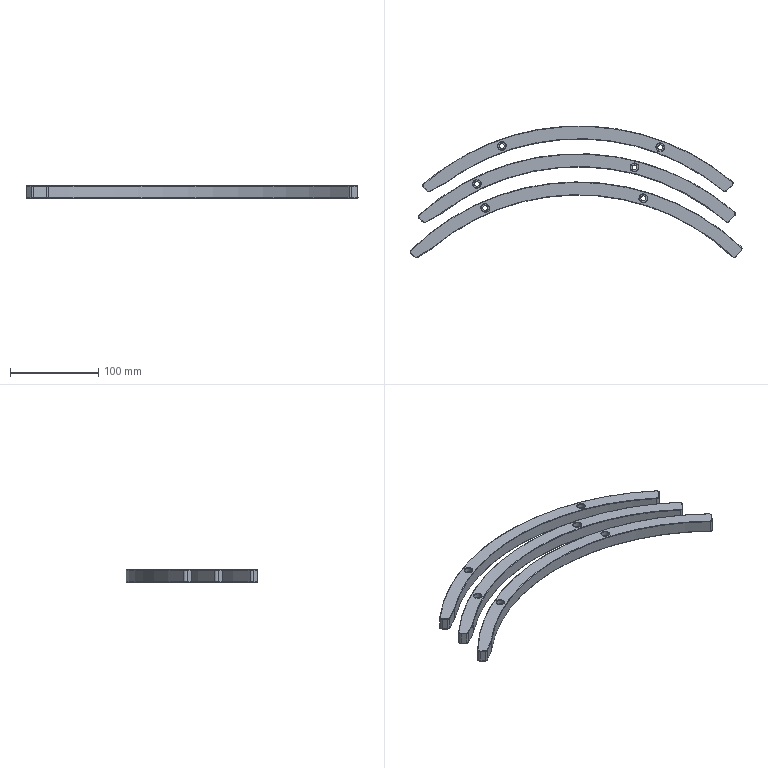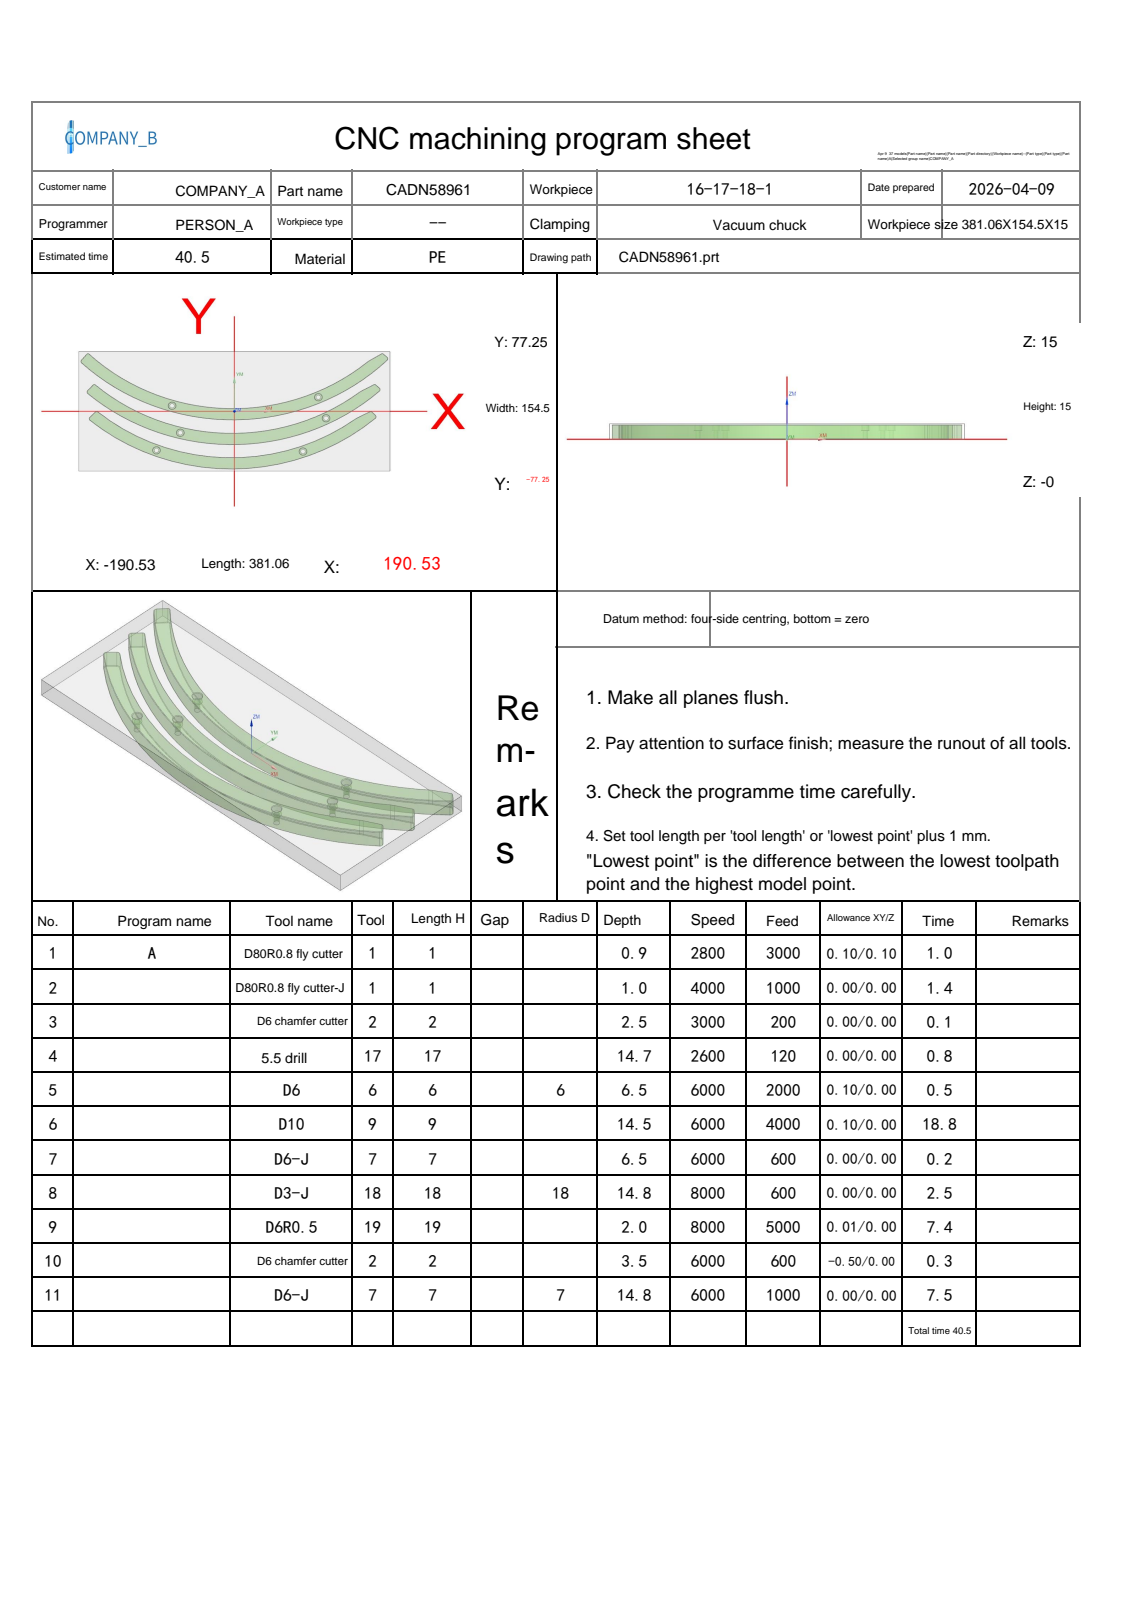NC program | NX | posted by the shop | part box 376.065 x 149.521 x 14 mm
Lines 2624 to 3929 of 3929:
N9 T19 M06
(D6R0.5  D=6. R=0.5 H=19 ce=0.01 di=0.00)
(MAX_Z=25. MIN_Z=13. Time=7.39M)
G00 G90 G54 X168.35 Y73.543 M03 S8000
G43 H19 Z25.
M08
Z14.484
G01 Z13.984 F5000.
X169.888 Y70.967
X178.897 Y76.346
G02 X181.043 Y76.938 I2.146 J-3.595
X183.776 Y75.923 I0.0 J-4.187
G01 X188.418 Y71.923
G02 X190.219 Y67.994 I-3.386 J-3.929
X188.662 Y64.289 I-5.187 J0.0
X-1.828 Y-13.478 I-190.491 J194.419
X-188.591 Y60.706 I0.0 J272.187
X-190.219 Y64.479 I3.559 J3.773
X-188.962 Y67.865 I5.187 J0.0
G01 X-182.395 Y75.485
G02 X-179.224 Y76.939 I3.172 J-2.733
X-176.334 Y75.781 I0.0 J-4.187
G03 X-1.828 Y5.895 I174.505 J182.927
X161.04 Y65.348 I0.0 J252.813
G02 X163.96 Y67.429 I14.293 J-16.969
G01 X169.888 Y70.967
X169.857 Y71.018 Z13.972
X169.834 Y71.058 Z13.959
X163.906 Y67.519
G03 X160.972 Y65.428 I11.427 J-19.14
G02 X-1.828 Y6.001 I-162.8 J193.281
X-176.257 Y75.854 I0.0 J252.708
G03 X-179.224 Y77.044 I-2.966 J-3.102
X-182.475 Y75.553 I0.0 J-4.292
G01 X-189.041 Y67.933
G03 X-190.324 Y64.479 I4.009 J-3.454
X-188.664 Y60.629 I5.292 J0.0
X-1.828 Y-13.583 I186.835 J198.079
X188.736 Y64.214 I0.0 J272.292
X190.324 Y67.994 I-3.704 J3.78
X188.487 Y72.003 I-5.292 J0.0
G01 X183.845 Y76.003
G03 X181.043 Y77.043 I-2.802 J-3.251
X178.843 Y76.437 I0.0 J-4.292
G01 X169.834 Y71.058
X169.806 Y71.103 Z13.942
X169.783 Y71.142 Z13.925
X178.793 Y76.521
G02 X181.043 Y77.142 I2.251 J-3.77
X183.909 Y76.077 I0.0 J-4.39
G01 X188.551 Y72.078
G02 X190.423 Y67.994 I-3.519 J-4.083
X188.805 Y64.144 I-5.39 J0.0
X-1.828 Y-13.682 I-190.633 J194.565
X-188.731 Y60.558 I0.0 J272.39
X-190.423 Y64.479 I3.699 J3.921
X-189.116 Y67.997 I5.39 J0.0
G01 X-182.55 Y75.618
G02 X-179.224 Y77.142 I3.326 J-2.866
X-176.193 Y75.929 I0.0 J-4.39
G03 X-1.828 Y6.099 I174.365 J182.78
X160.909 Y65.503 I0.0 J252.61
G02 X163.856 Y67.603 I14.425 J-17.125
G01 X169.783 Y71.142
X169.758 Y71.184 Z13.903
X169.736 Y71.221 Z13.881
X163.808 Y67.683
G03 X160.849 Y65.574 I11.525 J-19.304
G02 X-1.828 Y6.191 I-162.678 J193.135
X-176.129 Y75.995 I0.0 J252.517
G03 X-179.224 Y77.235 I-3.094 J-3.244
X-182.62 Y75.678 I0.0 J-4.483
G01 X-189.186 Y68.058
G03 X-190.515 Y64.479 I4.153 J-3.579
X-188.794 Y60.49 I5.483 J0.0
X-1.828 Y-13.774 I186.966 J198.218
X188.869 Y64.078 I0.0 J272.483
X190.515 Y67.994 I-3.837 J3.916
X188.611 Y72.148 I-5.483 J0.0
G01 X183.969 Y76.147
G03 X181.043 Y77.234 I-2.926 J-3.396
X178.745 Y76.6 I0.0 J-4.483
G01 X169.736 Y71.221
X169.712 Y71.261 Z13.855
X169.691 Y71.296 Z13.829
X178.701 Y76.675
G02 X181.043 Y77.321 I2.342 J-3.924
X184.026 Y76.213 I0.0 J-4.57
G01 X188.668 Y72.214
G02 X190.602 Y67.994 I-3.636 J-4.219
X188.93 Y64.016 I-5.57 J0.0
X-1.828 Y-13.861 I-190.759 J194.693
X-188.854 Y60.427 I0.0 J272.57
X-190.602 Y64.479 I3.822 J4.052
X-189.252 Y68.115 I5.57 J0.0
G01 X-182.685 Y75.735
G02 X-179.224 Y77.322 I3.462 J-2.983
X-176.069 Y76.058 I0.0 J-4.57
G03 X-1.828 Y6.278 I174.241 J182.65
X160.793 Y65.641 I0.0 J252.43
G02 X163.764 Y67.757 I14.54 J-17.262
G01 X169.691 Y71.296
X169.669 Y71.333 Z13.798
X169.65 Y71.366 Z13.768
X163.722 Y67.827
G03 X160.741 Y65.703 I11.611 J-19.448
G02 X-1.828 Y6.359 I-162.57 J193.006
X-176.014 Y76.117 I0.0 J252.35
G03 X-179.224 Y77.402 I-3.21 J-3.365
X-182.747 Y75.788 I0.0 J-4.65
G01 X-189.313 Y68.167
G03 X-190.683 Y64.479 I4.281 J-3.688
X-188.91 Y60.368 I5.65 J0.0
X-1.828 Y-13.942 I187.081 J198.34
X188.987 Y63.958 I0.0 J272.65
X190.683 Y67.994 I-3.954 J4.036
X188.721 Y72.275 I-5.65 J0.0
G01 X184.079 Y76.274
G03 X181.043 Y77.402 I-3.036 J-3.523
X178.659 Y76.744 I0.0 J-4.65
G01 X169.65 Y71.366
X169.63 Y71.399 Z13.734
X169.612 Y71.429 Z13.7
X178.622 Y76.808
G02 X181.043 Y77.476 I2.422 J-4.057
X184.127 Y76.331 I0.0 J-4.724
G01 X188.769 Y72.331
G02 X190.757 Y67.994 I-3.737 J-4.337
X189.039 Y63.905 I-5.724 J0.0
X-1.828 Y-14.016 I-190.867 J194.803
X-188.96 Y60.314 I0.0 J272.724
X-190.757 Y64.479 I3.928 J4.164
X-189.369 Y68.216 I5.724 J0.0
G01 X-182.803 Y75.836
G02 X-179.224 Y77.476 I3.579 J-3.084
X-175.963 Y76.17 I0.0 J-4.724
G03 X-1.828 Y6.433 I174.134 J182.538
X160.694 Y65.759 I0.0 J252.276
G02 X163.685 Y67.89 I14.639 J-17.381
G01 X169.612 Y71.429
X169.594 Y71.459 Z13.662
X169.578 Y71.486 Z13.624
X163.65 Y67.948
G03 X160.651 Y65.81 I11.683 J-19.569
G02 X-1.828 Y6.5 I-162.479 J192.899
X-175.917 Y76.219 I0.0 J252.209
G03 X-179.224 Y77.543 I-3.307 J-3.467
X-182.853 Y75.879 I0.0 J-4.791
G01 X-189.419 Y68.259
G03 X-190.824 Y64.479 I4.387 J-3.78
X-189.006 Y60.266 I5.791 J0.0
X-1.828 Y-14.082 I187.178 J198.443
X189.085 Y63.858 I0.0 J272.791
X190.824 Y67.994 I-4.053 J4.136
X188.813 Y72.381 I-5.791 J0.0
G01 X184.171 Y76.381
G03 X181.043 Y77.543 I-3.128 J-3.63
X178.587 Y76.865 I0.0 J-4.791
G01 X169.578 Y71.486
X169.562 Y71.513 Z13.584
X169.548 Y71.537 Z13.543
X178.557 Y76.916
G02 X181.043 Y77.601 I2.486 J-4.164
X184.209 Y76.425 I0.0 J-4.85
G01 X188.851 Y72.426
G02 X190.882 Y67.994 I-3.819 J-4.432
X189.126 Y63.816 I-5.85 J0.0
X-1.828 Y-14.141 I-190.955 J194.893
X-189.046 Y60.223 I0.0 J272.85
X-190.882 Y64.479 I4.014 J4.255
X-189.464 Y68.297 I5.85 J0.0
G01 X-182.898 Y75.918
G02 X-179.224 Y77.602 I3.674 J-3.166
X-175.876 Y76.261 I0.0 J-4.85
G03 X-1.828 Y6.559 I174.048 J182.448
X160.613 Y65.855 I0.0 J252.15
G02 X163.62 Y67.998 I14.72 J-17.476
G01 X169.548 Y71.537
X169.534 Y71.559 Z13.499
X169.522 Y71.58 Z13.456
X163.594 Y68.041
G03 X160.58 Y65.893 I11.739 J-19.662
G02 X-1.828 Y6.609 I-162.409 J192.815
X-175.841 Y76.297 I0.0 J252.1
G03 X-179.224 Y77.652 I-3.382 J-3.545
X-182.936 Y75.95 I0.0 J-4.9
G01 X-189.502 Y68.33
G03 X-190.932 Y64.479 I4.47 J-3.851
X-189.081 Y60.187 I5.9 J0.0
X-1.828 Y-14.191 I187.252 J198.522
X189.162 Y63.78 I0.0 J272.9
X190.932 Y67.994 I-4.129 J4.214
X188.884 Y72.464 I-5.9 J0.0
G01 X184.242 Y76.463
G03 X181.043 Y77.651 I-3.199 J-3.712
X178.532 Y76.959 I0.0 J-4.9
G01 X169.522 Y71.58
X169.511 Y71.599 Z13.41
X169.501 Y71.615 Z13.365
X178.51 Y76.994
G02 X181.043 Y77.693 I2.533 J-4.243
X184.269 Y76.495 I0.0 J-4.941
G01 X188.911 Y72.495
G02 X190.974 Y67.994 I-3.878 J-4.501
X189.19 Y63.75 I-5.941 J0.0
X-1.828 Y-14.232 I-191.019 J194.958
X-189.109 Y60.157 I0.0 J272.941
X-190.974 Y64.479 I4.077 J4.322
X-189.533 Y68.357 I5.941 J0.0
G01 X-182.967 Y75.977
G02 X-179.224 Y77.693 I3.743 J-3.225
X-175.813 Y76.327 I0.0 J-4.941
G03 X-1.828 Y6.65 I173.985 J182.382
X160.554 Y65.925 I0.0 J252.059
G02 X163.573 Y68.076 I14.779 J-17.546
G01 X169.501 Y71.615
X169.492 Y71.629 Z13.319
X169.485 Y71.641 Z13.274
X163.558 Y68.103
G03 X160.534 Y65.948 I11.776 J-19.724
G02 X-1.828 Y6.681 I-162.363 J192.76
X-175.792 Y76.349 I0.0 J252.028
G03 X-179.224 Y77.724 I-3.432 J-3.597
X-182.99 Y75.997 I0.0 J-4.972
G01 X-189.556 Y68.377
G03 X-191.004 Y64.479 I4.524 J-3.898
X-189.13 Y60.135 I5.972 J0.0
X-1.828 Y-14.263 I187.302 J198.574
X189.212 Y63.728 I0.0 J272.972
X191.004 Y67.994 I-4.179 J4.266
X188.931 Y72.518 I-5.972 J0.0
G01 X184.289 Y76.518
G03 X181.043 Y77.723 I-3.245 J-3.766
X178.495 Y77.02 I0.0 J-4.972
G01 X169.485 Y71.641
X169.479 Y71.652 Z13.228
X169.474 Y71.66 Z13.182
X178.484 Y77.039
G02 X181.043 Y77.745 I2.56 J-4.287
X184.303 Y76.534 I0.0 J-4.993
G01 X188.945 Y72.534
G02 X191.026 Y67.994 I-3.912 J-4.54
X189.227 Y63.713 I-5.993 J0.0
X-1.828 Y-14.285 I-191.055 J194.995
X-189.145 Y60.119 I0.0 J272.993
X-191.026 Y64.479 I4.112 J4.36
X-189.573 Y68.391 I5.993 J0.0
G01 X-183.006 Y76.011
G02 X-179.224 Y77.745 I3.783 J-3.259
X-175.777 Y76.365 I0.0 J-4.993
G03 X-1.828 Y6.702 I173.949 J182.344
X160.52 Y65.965 I0.0 J252.007
G02 X163.547 Y68.121 I14.813 J-17.586
G01 X169.474 Y71.66
X169.47 Y71.666 Z13.137
X169.468 Y71.671 Z13.091
X163.54 Y68.132
G03 X160.512 Y65.974 I11.793 J-19.753
G02 X-1.828 Y6.715 I-162.341 J192.734
X-175.768 Y76.374 I0.0 J251.994
G03 X-179.224 Y77.758 I-3.455 J-3.622
X-183.016 Y76.02 I0.0 J-5.006
G01 X-189.582 Y68.399
G03 X-191.038 Y64.479 I4.55 J-3.92
X-189.153 Y60.11 I6.006 J0.0
X-1.828 Y-14.297 I187.325 J198.599
X189.236 Y63.704 I0.0 J273.006
X191.038 Y67.994 I-4.203 J4.29
X188.953 Y72.544 I-6.006 J0.0
G01 X184.311 Y76.544
G03 X181.043 Y77.757 I-3.268 J-3.792
X178.477 Y77.05 I0.0 J-5.006
G01 X169.468 Y71.671
X169.465 Y71.674 Z13.
X178.476 Y77.054
G02 X179.504 Y77.519 I2.592 J-4.356
X179.713 Y77.582 I1.539 J-4.768
X181.042 Y77.761 I1.329 J-4.834
X184.314 Y76.547 I0.0 J-5.014
G01 X188.787 Y72.692
X189.178 Y72.346
G02 X191.042 Y67.994 I-4.148 J-4.352
X190.464 Y65.422 I-6.013 J0.0
X190.12 Y64.794 I-6.048 J2.91
X189.246 Y63.708 I-5.151 J3.252
X-1.842 Y-14.305 I-191.088 J195.02
X-26.922 Y-13.151 I0.0 J273.034
G01 X-26.934 Y-13.143
X-27.069 Y-13.131
X-30.191 Y-12.824
X-30.437 Y-12.798
X-33.554 Y-12.452
X-36.387 Y-12.105
G02 X-69.081 Y-5.894 I34.769 J272.19
G01 X-69.394 Y-5.808
G02 X-88.032 Y-.339 I68.396 J267.567
G01 X-88.052 Y-.327
X-89.862 Y.282
X-90.101 Y.363
X-91.104 Y.709
X-91.108
G02 X-100.542 Y4.167 I92.07 J265.779
X-109.05 Y7.635 I103.191 J265.362
X-129.387 Y17.331 I107.517 J251.692
X-189.156 Y60.107 I127.592 J241.425
X-190.121 Y61.28 I4.155 J4.397
X-191.042 Y64.479 I5.088 J3.199
X-190.392 Y67.199 I6.01 J0.0
X-189.585 Y68.402 I5.359 J-2.72
G01 X-183.019 Y76.022
G02 X-182.148 Y76.82 I3.795 J-3.27
G01 X-182.059 Y76.882
G02 X-179.224 Y77.762 I2.836 J-4.132
X-175.765 Y76.377 I0.0 J-5.011
G01 X-173.359 Y74.112
X-172.985 Y73.765
G03 X-1.828 Y6.719 I171.157 J184.944
X157.334 Y63.347 I0.0 J251.99
G01 X157.758 Y63.694
X160.63 Y66.078
G02 X163.538 Y68.135 I14.739 J-17.743
G01 X169.465 Y71.674
G00 Z25.
X159.122 Y34.303
Z14.484
G01 Z13.984
X160.545 Y31.663
X169.783 Y36.641
G02 X171.769 Y37.142 I1.986 J-3.686
X174.639 Y36.004 I0.0 J-4.187
G01 X179.1 Y31.804
G02 X180.732 Y28.027 I-3.555 J-3.777
X179.009 Y24.167 I-5.187 J0.0
X-2.761 Y-45.424 I-181.77 J202.596
X-180.995 Y21.049 I0.0 J272.187
X-182.786 Y24.969 I3.396 J3.92
X-181.376 Y28.524 I5.187 J0.0
G01 X-174.544 Y35.782
G02 X-171.495 Y37.099 I3.049 J-2.87
X-168.746 Y36.07 I0.0 J-4.187
G03 X-2.761 Y-26.051 I165.985 J190.692
X151.46 Y26.437 I0.0 J252.813
G02 X154.468 Y28.387 I13.535 J-17.58
G01 X160.545 Y31.663
X160.518 Y31.714 Z13.972
X160.496 Y31.755 Z13.959
X154.419 Y28.48
G03 X151.395 Y26.52 I10.576 J-19.624
G02 X-2.761 Y-25.945 I-154.157 J200.243
X-168.677 Y36.15 I0.0 J252.708
G03 X-171.495 Y37.204 I-2.818 J-3.237
X-174.62 Y35.854 I0.0 J-4.292
G01 X-181.452 Y28.596
G03 X-182.891 Y24.969 I3.853 J-3.627
X-181.064 Y20.969 I5.292 J0.0
X-2.761 Y-45.529 I178.303 J205.794
X179.079 Y24.088 I0.0 J272.292
X180.837 Y28.027 I-3.534 J3.939
X179.172 Y31.881 I-5.292 J0.0
G01 X174.711 Y36.08
G03 X171.769 Y37.247 I-2.942 J-3.125
X169.733 Y36.733 I0.0 J-4.292
G01 X160.496 Y31.755
X160.47 Y31.802 Z13.942
X160.449 Y31.842 Z13.925
X169.686 Y36.82
G02 X171.769 Y37.345 I2.083 J-3.865
X174.778 Y36.152 I0.0 J-4.39
G01 X179.24 Y31.952
G02 X180.935 Y28.027 I-3.694 J-3.925
X179.145 Y24.015 I-5.39 J0.0
X-2.761 Y-45.628 I-181.906 J202.748
X-181.128 Y20.895 I0.0 J272.39
X-182.989 Y24.969 I3.53 J4.074
X-181.524 Y28.663 I5.39 J0.0
G01 X-174.692 Y35.921
G02 X-171.495 Y37.303 I3.197 J-3.009
X-168.613 Y36.224 I0.0 J-4.39
G03 X-2.761 Y-25.847 I165.851 J190.539
X151.335 Y26.598 I0.0 J252.61
G02 X154.372 Y28.567 I13.659 J-17.742
G01 X160.449 Y31.842
X160.426 Y31.885 Z13.903
X160.405 Y31.923 Z13.881
X154.328 Y28.648
G03 X151.279 Y26.671 I10.666 J-19.792
G02 X-2.761 Y-25.755 I-154.04 J200.091
X-168.552 Y36.294 I0.0 J252.517
G03 X-171.495 Y37.395 I-2.943 J-3.381
X-174.759 Y35.985 I0.0 J-4.483
G01 X-181.591 Y28.727
G03 X-183.082 Y24.969 I3.992 J-3.758
X-181.189 Y20.825 I5.483 J0.0
X-2.761 Y-45.72 I178.428 J205.938
X179.207 Y23.946 I0.0 J272.483
X181.028 Y28.027 I-3.661 J4.081
X179.303 Y32.02 I-5.483 J0.0
G01 X174.841 Y36.219
G03 X171.769 Y37.438 I-3.073 J-3.264
X169.642 Y36.901 I0.0 J-4.483
G01 X160.405 Y31.923
X160.383 Y31.964 Z13.855
X160.364 Y32. Z13.829
X169.601 Y36.978
G02 X171.769 Y37.525 I2.168 J-4.023
X174.901 Y36.283 I0.0 J-4.57
G01 X179.363 Y32.083
G02 X181.115 Y28.027 I-3.817 J-4.056
X179.265 Y23.882 I-5.57 J0.0
X-2.761 Y-45.807 I-182.026 J202.881
X-181.246 Y20.759 I0.0 J272.57
X-183.169 Y24.969 I3.647 J4.21
X-181.654 Y28.786 I5.57 J0.0
G01 X-174.822 Y36.044
G02 X-171.495 Y37.482 I3.327 J-3.132
X-168.495 Y36.359 I0.0 J-4.57
G03 X-2.761 Y-25.668 I165.733 J190.404
X151.226 Y26.74 I0.0 J252.43
G02 X154.287 Y28.725 I13.768 J-17.884
G01 X160.364 Y32.
X160.344 Y32.037 Z13.798
X160.325 Y32.071 Z13.768
X154.248 Y28.796
G03 X151.177 Y26.804 I10.746 J-19.939
G02 X-2.761 Y-25.587 I-153.938 J199.958
X-168.442 Y36.42 I0.0 J252.35
G03 X-171.495 Y37.563 I-3.053 J-3.508
X-174.881 Y36.1 I0.0 J-4.65
G01 X-181.713 Y28.842
G03 X-183.249 Y24.969 I4.114 J-3.873
X-181.299 Y20.698 I5.65 J0.0
X-2.761 Y-45.888 I178.538 J206.065
X179.319 Y23.822 I0.0 J272.65
X181.196 Y28.027 I-3.774 J4.206
X179.418 Y32.142 I-5.65 J0.0
G01 X174.956 Y36.341
G03 X171.769 Y37.606 I-3.187 J-3.386
X169.563 Y37.049 I0.0 J-4.65
G01 X160.325 Y32.071
X160.307 Y32.105 Z13.734
X160.29 Y32.136 Z13.7
X169.527 Y37.114
G02 X171.769 Y37.68 I2.241 J-4.159
X175.007 Y36.395 I0.0 J-4.724
G01 X179.469 Y32.196
G02 X181.27 Y28.027 I-3.924 J-4.168
X179.368 Y23.766 I-5.724 J0.0
X-2.761 Y-45.962 I-182.13 J202.996
X-181.347 Y20.642 I0.0 J272.724
X-183.323 Y24.969 I3.748 J4.327
X-181.767 Y28.892 I5.724 J0.0
G01 X-174.935 Y36.15
G02 X-171.495 Y37.637 I3.44 J-3.238
X-168.393 Y36.476 I0.0 J-4.724
G03 X-2.761 Y-25.513 I165.632 J190.287
X151.132 Y26.863 I0.0 J252.276
G02 X154.213 Y28.861 I13.862 J-18.007
G01 X160.29 Y32.136
X160.274 Y32.167 Z13.662
X160.259 Y32.195 Z13.624
X154.182 Y28.919
G03 X151.091 Y26.916 I10.813 J-20.063
G02 X-2.761 Y-25.446 I-153.853 J199.847
X-168.349 Y36.526 I0.0 J252.209
G03 X-171.495 Y37.703 I-3.146 J-3.614
X-174.984 Y36.196 I0.0 J-4.791
G01 X-181.816 Y28.938
G03 X-183.39 Y24.969 I4.217 J-3.969
X-181.391 Y20.592 I5.791 J0.0
X-2.761 Y-46.028 I178.63 J206.171
X179.413 Y23.717 I0.0 J272.791
X181.336 Y28.027 I-3.867 J4.31
X179.514 Y32.244 I-5.791 J0.0
G01 X175.053 Y36.444
G03 X171.769 Y37.746 I-3.284 J-3.489
X169.496 Y37.173 I0.0 J-4.791
G01 X160.259 Y32.195
X160.244 Y32.222 Z13.584
X160.231 Y32.246 Z13.543
X169.468 Y37.224
G02 X171.769 Y37.805 I2.301 J-4.269
X175.093 Y36.487 I0.0 J-4.85
G01 X179.555 Y32.287
G02 X181.395 Y28.027 I-4.009 J-4.26
X179.452 Y23.673 I-5.85 J0.0
X-2.761 Y-46.087 I-182.213 J203.09
X-181.429 Y20.547 I0.0 J272.85
X-183.449 Y24.969 I3.831 J4.421
X-181.858 Y28.978 I5.85 J0.0
G01 X-175.026 Y36.236
G02 X-171.495 Y37.762 I3.531 J-3.324
X-168.311 Y36.57 I0.0 J-4.85
G03 X-2.761 Y-25.388 I165.549 J190.192
X151.055 Y26.962 I0.0 J252.15
G02 X154.154 Y28.971 I13.939 J-18.106
G01 X160.231 Y32.246
X160.218 Y32.27 Z13.499
X160.207 Y32.29 Z13.456
X154.13 Y29.015
G03 X151.025 Y27.002 I10.864 J-20.159
G02 X-2.761 Y-25.337 I-153.786 J199.761
X-168.278 Y36.608 I0.0 J252.1
G03 X-171.495 Y37.812 I-3.217 J-3.696
X-175.063 Y36.271 I0.0 J-4.9
G01 X-181.895 Y29.012
G03 X-183.499 Y24.969 I4.296 J-4.044
X-181.462 Y20.51 I5.9 J0.0
X-2.761 Y-46.137 I178.701 J206.253
X179.485 Y23.636 I0.0 J272.9
X181.445 Y28.027 I-3.94 J4.392
X179.589 Y32.323 I-5.9 J0.0
G01 X175.127 Y36.523
G03 X171.769 Y37.855 I-3.358 J-3.568
X169.444 Y37.269 I0.0 J-4.9
G01 X160.207 Y32.29
X160.197 Y32.31 Z13.41
X160.188 Y32.327 Z13.365
X169.425 Y37.305
G02 X171.769 Y37.896 I2.344 J-4.35
X175.156 Y36.553 I0.0 J-4.941
G01 X179.617 Y32.353
G02 X181.486 Y28.027 I-4.072 J-4.326
X179.513 Y23.605 I-5.941 J0.0
X-2.761 Y-46.178 I-182.274 J203.158
X-181.489 Y20.478 I0.0 J272.941
X-183.54 Y24.969 I3.89 J4.49
X-181.925 Y29.041 I5.941 J0.0
G01 X-175.093 Y36.299
G02 X-171.495 Y37.853 I3.598 J-3.387
X-168.251 Y36.639 I0.0 J-4.941
G03 X-2.761 Y-25.296 I165.489 J190.123
X151. Y27.035 I0.0 J252.059
G02 X154.11 Y29.052 I13.995 J-18.178
G01 X160.188 Y32.327
X160.18 Y32.341 Z13.319
X160.173 Y32.354 Z13.274
X154.096 Y29.079
G03 X150.981 Y27.059 I10.898 J-20.222
G02 X-2.761 Y-25.265 I-153.742 J199.704
X-168.231 Y36.662 I0.0 J252.028
G03 X-171.495 Y37.884 I-3.264 J-3.75
X-175.115 Y36.32 I0.0 J-4.972
G01 X-181.947 Y29.062
G03 X-183.571 Y24.969 I4.348 J-4.093
X-181.509 Y20.455 I5.972 J0.0
X-2.761 Y-46.209 I178.748 J206.308
X179.533 Y23.582 I0.0 J272.972
X181.517 Y28.027 I-3.988 J4.445
X179.638 Y32.376 I-5.972 J0.0
G01 X175.177 Y36.575
G03 X171.769 Y37.927 I-3.408 J-3.62
X169.41 Y37.332 I0.0 J-4.972
G01 X160.173 Y32.354
X160.167 Y32.364 Z13.228
X160.163 Y32.373 Z13.182
X169.4 Y37.351
G02 X171.769 Y37.948 I2.369 J-4.396
X175.191 Y36.591 I0.0 J-4.993
G01 X179.653 Y32.391
G02 X181.538 Y28.027 I-4.108 J-4.364
X179.548 Y23.566 I-5.993 J0.0
X-2.761 Y-46.231 I-182.309 J203.196
X-181.523 Y20.439 I0.0 J272.993
X-183.592 Y24.969 I3.924 J4.53
X-181.963 Y29.076 I5.993 J0.0
G01 X-175.131 Y36.335
G02 X-171.495 Y37.906 I3.636 J-3.422
X-168.217 Y36.679 I0.0 J-4.993
G03 X-2.761 Y-25.244 I165.455 J190.084
X150.968 Y27.076 I0.0 J252.007
G02 X154.086 Y29.097 I14.026 J-18.22
G01 X160.163 Y32.373
X160.159 Y32.379 Z13.137
X160.157 Y32.384 Z13.091
X154.08 Y29.109
G03 X150.96 Y27.086 I10.914 J-20.252
G02 X-2.761 Y-25.231 I-153.722 J199.677
X-168.208 Y36.688 I0.0 J251.994
G03 X-171.495 Y37.918 I-3.287 J-3.776
X-175.14 Y36.343 I0.0 J-5.006
G01 X-181.972 Y29.085
G03 X-183.605 Y24.969 I4.373 J-4.116
X-181.532 Y20.429 I6.006 J0.0
X-2.761 Y-46.243 I178.77 J206.333
X179.556 Y23.557 I0.0 J273.006
X181.551 Y28.027 I-4.011 J4.47
X179.662 Y32.401 I-6.006 J0.0
G01 X175.2 Y36.6
G03 X171.769 Y37.961 I-3.431 J-3.645
X169.394 Y37.362 I0.0 J-5.006
G01 X160.157 Y32.384
X160.155 Y32.387 Z13.
X163.642 Y34.267
X169.392 Y37.365
G02 X171.769 Y37.965 I2.377 J-4.41
X175.203 Y36.603 I0.0 J-5.01
G01 X179.664 Y32.404
X179.882 Y32.188
G02 X181.555 Y28.027 I-4.337 J-4.16
X180.882 Y25.263 I-6.01 J0.0
X179.559 Y23.554 I-5.359 J2.782
X-2.761 Y-46.247 I-182.32 J203.211
X-181.534 Y20.426 I0.0 J273.012
G01 X-181.795 Y20.666
G02 X-183.609 Y24.969 I4.196 J4.303
X-183.181 Y27.196 I6.01 J0.0
X-181.976 Y29.087 I5.617 J-2.25
G01 X-175.142 Y36.348
G02 X-171.495 Y37.922 I3.647 J-3.437
X-168.206 Y36.691 I0.0 J-5.011
G03 X-159.94 Y29.801 I165.385 J190.
X-79.802 Y-13.162 I157.179 J196.961
G01 X-79.456 Y-13.273
X-76.68 Y-14.142
X-75.986 Y-14.354
G03 X-68.354 Y-16.541 I73.225 J241.116
G01 X-66.82 Y-16.949
G03 X-53.089 Y-20.15 I64.058 J243.712
G01 X-50.661 Y-20.633
X-50.314 Y-20.7
G03 X-34.008 Y-23.282 I47.552 J247.463
G01 X-31.958 Y-23.53
G03 X-18.049 Y-24.763 I29.196 J250.293
G01 X-15.262 Y-24.917
X-14.927 Y-24.933
G03 X-2.761 Y-25.227 I12.166 J251.696
X55.726 Y-18.346 I0.0 J251.99
G01 X56.195 Y-18.233
X58.971 Y-17.549
G03 X143.973 Y21.902 I-61.732 J244.311
G01 X144.32 Y22.151
X146.749 Y23.919
X147.096 Y24.175
X147.168 Y24.228
G03 X150.949 Y27.083 I-149.809 J202.372
G02 X154.035 Y29.089 I14.114 J-18.335
G01 X160.155 Y32.387
G00 Z25.
X154.371 Y-.399
Z14.484
G01 Z13.984
X155.74 Y-3.068
X165.064 Y1.716
G02 X166.978 Y2.179 I1.914 J-3.724
X169.925 Y.966 I0.0 J-4.187
G01 X174.28 Y-3.349
G02 X175.815 Y-7.033 I-3.651 J-3.684
X174.014 Y-10.963 I-5.187 J0.0
X-3.645 Y-76.939 I-177.659 J206.211
X-178.27 Y-13.538 I0.0 J272.187
X-180.13 Y-9.559 I3.327 J3.979
X-178.627 Y-5.908 I5.187 J0.0
G01 X-172.268 Y.508
G02 X-168.584 Y2.044 I3.684 J-3.651
X-165.268 Y.845 I0.0 J-5.187
G03 X-3.645 Y-57.565 I161.623 J194.403
X146.563 Y-8.104 I0.0 J252.813
G02 X149.616 Y-6.211 I13.182 J-17.846
G01 X155.74 Y-3.068
X155.713 Y-3.016 Z13.972
X155.692 Y-2.975 Z13.959
X149.568 Y-6.117
G03 X146.5 Y-8.02 I10.177 J-19.833
G02 X-3.645 Y-57.46 I-150.146 J203.268
X-165.201 Y.926 I0.0 J252.708
G03 X-168.584 Y2.149 I-3.383 J-4.069
X-172.343 Y.582 I0.0 J-5.292
G01 X-178.702 Y-5.834
G03 X-180.235 Y-9.559 I3.759 J-3.725
X-178.338 Y-13.618 I5.292 J0.0
X-3.645 Y-77.044 I174.693 J208.866
X174.083 Y-11.042 I0.0 J272.292
X175.92 Y-7.033 I-3.454 J4.009
X174.354 Y-3.274 I-5.292 J0.0
G01 X169.999 Y1.041
G03 X166.978 Y2.284 I-3.021 J-3.048
X165.021 Y1.812 I0.0 J-4.292
G01 X155.692 Y-2.975
X155.668 Y-2.927 Z13.942
X155.647 Y-2.887 Z13.925
X164.977 Y1.9
G02 X166.978 Y2.383 I2.001 J-3.908
X170.069 Y1.111 I0.0 J-4.39
G01 X174.423 Y-3.205
G02 X176.019 Y-7.033 I-3.794 J-3.829
X174.147 Y-11.117 I-5.39 J0.0
X-3.645 Y-77.142 I-177.792 J206.365
X-178.401 Y-13.694 I0.0 J272.39
X-180.333 Y-9.559 I3.458 J4.135
X-178.771 Y-5.765 I5.39 J0.0
G01 X-172.413 Y.651
G02 X-168.584 Y2.247 I3.829 J-3.794
X-165.132 Y.996 I0.0 J-5.39
G03 X-3.645 Y-57.362 I161.487 J194.252
X146.442 Y-7.94 I0.0 J252.61
G02 X149.525 Y-6.029 I13.303 J-18.01
G01 X155.647 Y-2.887
X155.625 Y-2.843 Z13.903
X155.605 Y-2.805 Z13.881
X149.484 Y-5.946
G03 X146.387 Y-7.866 I10.262 J-20.004
G02 X-3.645 Y-57.269 I-150.032 J203.114
X-165.079 Y1.073 I0.0 J252.517
G03 X-168.584 Y2.34 I-3.505 J-4.216
X-172.478 Y.716 I0.0 J-5.483
G01 X-178.837 Y-5.7
G03 X-180.426 Y-9.559 I3.894 J-3.859
X-178.461 Y-13.765 I5.483 J0.0
X-3.645 Y-77.235 I174.815 J209.013
X174.207 Y-11.187 I0.0 J272.483
X176.111 Y-7.033 I-3.579 J4.154
X174.488 Y-3.139 I-5.483 J0.0
G01 X170.134 Y1.177
G03 X166.978 Y2.475 I-3.156 J-3.184
X164.935 Y1.983 I0.0 J-4.483
G01 X155.605 Y-2.805
X155.584 Y-2.764 Z13.855
X155.565 Y-2.727 Z13.829
X164.896 Y2.06
G02 X166.978 Y2.562 I2.082 J-4.068
X170.195 Y1.238 I0.0 J-4.57
G01 X174.549 Y-3.077
G02 X176.198 Y-7.033 I-3.921 J-3.956
X174.264 Y-11.253 I-5.57 J0.0
X-3.645 Y-77.322 I-177.909 J206.501
X-178.516 Y-13.832 I0.0 J272.57
X-180.513 Y-9.559 I3.573 J4.272
X-178.899 Y-5.639 I5.57 J0.0
G01 X-172.54 Y.777
G02 X-168.584 Y2.427 I3.956 J-3.921
X-165.023 Y1.14 I0.0 J-5.57
G03 X-3.645 Y-57.182 I161.378 J194.108
X146.336 Y-7.796 I0.0 J252.43
G02 X149.438 Y-5.871 I13.41 J-18.154
G01 X155.565 Y-2.727
X155.546 Y-2.689 Z13.798
X155.529 Y-2.655 Z13.768
X149.401 Y-5.799
G03 X146.287 Y-7.731 I10.344 J-20.151
G02 X-3.645 Y-57.102 I-149.932 J202.979
X-164.972 Y1.202 I0.0 J252.35
G03 X-168.584 Y2.507 I-3.612 J-4.345
X-172.598 Y.834 I0.0 J-5.65
G01 X-178.956 Y-5.582
G03 X-180.593 Y-9.559 I4.013 J-3.978
X-178.568 Y-13.894 I5.65 J0.0
X-3.645 Y-77.402 I174.923 J209.142
X174.317 Y-11.314 I0.0 J272.65
X176.279 Y-7.033 I-3.688 J4.281
X174.606 Y-3.02 I-5.65 J0.0
G01 X170.252 Y1.296
G03 X166.978 Y2.643 I-3.274 J-3.303
X164.853 Y2.129 I0.0 J-4.65
G01 X155.529 Y-2.655
X155.511 Y-2.621 Z13.734
X155.495 Y-2.59 Z13.7
X164.822 Y2.196
G02 X166.978 Y2.717 I2.156 J-4.204
X170.304 Y1.348 I0.0 J-4.724
G01 X174.658 Y-2.967
G02 X176.353 Y-7.033 I-4.03 J-4.066
X174.365 Y-11.37 I-5.724 J0.0
X-3.645 Y-77.476 I-178.01 J206.618
X-178.616 Y-13.95 I0.0 J272.724
X-180.667 Y-9.559 I3.673 J4.391
X-179.009 Y-5.53 I5.724 J0.0
G01 X-172.65 Y.886
G02 X-168.584 Y2.581 I4.066 J-4.03
X-164.925 Y1.259 I0.0 J-5.724
G03 X-3.645 Y-57.027 I161.279 J193.989
X146.244 Y-7.671 I0.0 J252.276
G02 X149.367 Y-5.734 I13.502 J-18.279
G01 X155.495 Y-2.59
X155.479 Y-2.558 Z13.662
X155.464 Y-2.53 Z13.624
X149.337 Y-5.674
G03 X146.204 Y-7.618 I10.408 J-20.276
G02 X-3.645 Y-56.961 I-149.849 J202.866
X-164.882 Y1.31 I0.0 J252.209
G03 X-168.584 Y2.648 I-3.702 J-4.453
X-172.698 Y.933 I0.0 J-5.791
G01 X-179.056 Y-5.483
G03 X-180.734 Y-9.559 I4.113 J-4.077
X-178.658 Y-14.001 I5.791 J0.0
X-3.645 Y-77.543 I175.013 J209.249
X174.409 Y-11.421 I0.0 J272.791
X176.42 Y-7.033 I-3.78 J4.387
X174.705 Y-2.92 I-5.791 J0.0
G01 X170.351 Y1.396
G03 X166.978 Y2.784 I-3.373 J-3.403
X164.794 Y2.257 I0.0 J-4.791
G01 X155.464 Y-2.53
X155.45 Y-2.503 Z13.584
X155.438 Y-2.478 Z13.543
X164.76 Y2.305
G02 X166.978 Y2.842 I2.218 J-4.313
X170.392 Y1.437 I0.0 J-4.85
G01 X174.746 Y-2.878
G02 X176.478 Y-7.033 I-4.118 J-4.155
X174.447 Y-11.465 I-5.85 J0.0
X-3.645 Y-77.602 I-178.092 J206.713
X-178.696 Y-14.046 I0.0 J272.85
X-180.793 Y-9.559 I3.753 J4.487
X-179.098 Y-5.441 I5.85 J0.0
G01 X-172.739 Y.975
G02 X-168.584 Y2.707 I4.155 J-4.118
X-164.844 Y1.355 I0.0 J-5.85
G03 X-3.645 Y-56.902 I161.199 J193.893
X146.169 Y-7.571 I0.0 J252.15
G02 X149.31 Y-5.622 I13.576 J-18.379
G01 X155.438 Y-2.478
X155.425 Y-2.455 Z13.499
X155.415 Y-2.433 Z13.456
X149.287 Y-5.578
G03 X146.139 Y-7.53 I10.458 J-20.372
G02 X-3.645 Y-56.852 I-149.784 J202.778
X-164.812 Y1.394 I0.0 J252.1
G03 X-168.584 Y2.757 I-3.772 J-4.537
X-172.775 Y1.01 I0.0 J-5.9
G01 X-179.134 Y-5.406
G03 X-180.843 Y-9.559 I4.191 J-4.153
X-178.728 Y-14.085 I5.9 J0.0
X-3.645 Y-77.652 I175.083 J209.333
X174.48 Y-11.503 I0.0 J272.9
X176.529 Y-7.033 I-3.851 J4.47
X174.782 Y-2.842 I-5.9 J0.0
G01 X170.427 Y1.473
G03 X166.978 Y2.893 I-3.449 J-3.48
X164.737 Y2.35 I0.0 J-4.9
G01 X155.415 Y-2.433
X155.405 Y-2.414 Z13.41
X155.396 Y-2.397 Z13.365
X164.718 Y2.387
G02 X166.978 Y2.934 I2.26 J-4.394
X170.456 Y1.502 I0.0 J-4.941
G01 X174.811 Y-2.813
G02 X176.57 Y-7.033 I-4.182 J-4.22
X174.506 Y-11.534 I-5.941 J0.0
X-3.645 Y-77.693 I-178.152 J206.782
X-178.755 Y-14.117 I0.0 J272.941
X-180.884 Y-9.559 I3.812 J4.557
X-179.163 Y-5.377 I5.941 J0.0
G01 X-172.804 Y1.039
G02 X-168.584 Y2.798 I4.22 J-4.182
X-164.786 Y1.425 I0.0 J-5.941
G03 X-3.645 Y-56.811 I161.141 J193.823
X146.115 Y-7.497 I0.0 J252.059
G02 X149.274 Y-5.538 I13.63 J-18.453
G01 X155.396 Y-2.397
X155.388 Y-2.382 Z13.319
X155.382 Y-2.37 Z13.274
X149.26 Y-5.511
G03 X146.097 Y-7.472 I10.485 J-20.439
G02 X-3.645 Y-56.78 I-149.742 J202.72
X-164.766 Y1.449 I0.0 J252.028
G03 X-168.584 Y2.829 I-3.818 J-4.592
X-172.826 Y1.061 I0.0 J-5.972
G01 X-179.185 Y-5.356
G03 X-180.915 Y-9.559 I4.242 J-4.204
X-178.774 Y-14.14 I5.972 J0.0
X-3.645 Y-77.724 I175.129 J209.388
X174.527 Y-11.557 I0.0 J272.972
X176.601 Y-7.033 I-3.898 J4.524
X174.832 Y-2.791 I-5.972 J0.0
G01 X170.478 Y1.524
G03 X166.978 Y2.965 I-3.5 J-3.531
X164.712 Y2.418 I0.0 J-4.972
G01 X155.382 Y-2.37
X155.376 Y-2.359 Z13.228
X155.372 Y-2.35 Z13.182
X164.701 Y2.437
G02 X166.978 Y2.986 I2.277 J-4.444
X170.493 Y1.539 I0.0 J-4.993
G01 X174.847 Y-2.776
G02 X176.622 Y-7.033 I-4.219 J-4.257
X174.54 Y-11.574 I-5.993 J0.0
X-3.645 Y-77.745 I-178.186 J206.822
X-178.788 Y-14.157 I0.0 J272.993
X-180.936 Y-9.559 I3.845 J4.597
X-179.2 Y-5.341 I5.993 J0.0
G01 X-172.841 Y1.076
G02 X-168.584 Y2.85 I4.257 J-4.219
X-164.753 Y1.465 I0.0 J-5.993
G03 X-3.645 Y-56.759 I161.108 J193.783
X146.084 Y-7.455 I0.0 J252.007
G02 X149.25 Y-5.492 I13.661 J-18.495
G01 X155.372 Y-2.35
X155.369 Y-2.344 Z13.137
X155.366 Y-2.339 Z13.091
X149.244 Y-5.481
G03 X146.077 Y-7.445 I10.501 J-20.469
G02 X-3.645 Y-56.746 I-149.722 J202.693
X-164.745 Y1.475 I0.0 J251.994
G03 X-168.584 Y2.863 I-3.84 J-4.618
X-172.85 Y1.084 I0.0 J-6.006
G01 X-179.209 Y-5.332
G03 X-180.949 Y-9.559 I4.266 J-4.228
X-178.796 Y-14.166 I6.006 J0.0
X-3.645 Y-77.758 I175.151 J209.414
X174.549 Y-11.583 I0.0 J273.006
X176.634 Y-7.033 I-3.92 J4.55
X174.856 Y-2.767 I-6.006 J0.0
G01 X170.502 Y1.548
G03 X166.978 Y2.998 I-3.524 J-3.556
X164.696 Y2.448 I0.0 J-5.006
G01 X155.366 Y-2.339
X155.364 Y-2.336 Z13.
X163.275 Y1.724
X164.689 Y2.449
G02 X166.978 Y3.002 I2.289 J-4.463
X169.292 Y2.436 I0.0 J-5.016
G01 X169.334 Y2.414
G02 X170.505 Y1.551 I-2.39 J-4.467
G01 X171.032 Y1.028
X174.873 Y-2.778
G02 X176.081 Y-4.506 I-4.2 J-4.224
X176.639 Y-7.033 I-5.453 J-2.528
X174.543 Y-11.594 I-6.01 J0.0
G03 X174.327 Y-11.779 I222.329 J-259.065
G02 X-3.645 Y-77.761 I-177.972 J207.029
X-178.806 Y-14.163 I0.0 J273.011
G01 X-179.019 Y-13.976
G02 X-180.953 Y-9.559 I4.076 J4.417
X-179.212 Y-5.329 I6.01 J0.0
G01 X-172.854 Y1.086
G02 X-171.881 Y1.882 I4.269 J-4.231
X-168.584 Y2.866 I3.297 J-5.029
X-164.8 Y1.526 I0.0 J-6.013
G01 X-164.742 Y1.478
G03 X-3.645 Y-56.742 I161.097 J193.77
X98.822 Y-34.968 I0.0 J251.99
G01 X100.601 Y-34.168
X100.948 Y-34.01
G03 X146.074 Y-7.442 I-104.593 J229.258
G02 X149.247 Y-5.474 I13.679 J-18.521
G01 X155.364 Y-2.336
G00 Z25.
G91 G28 Z0.0
M05
M09
G91 G28 Z0.0
M01
N10 T02 M06
(D6 chamfer cutter  D=6. R=0. H=02 ce=-0.50 di=0.00)
(MAX_Z=34. MIN_Z=11.5 Time=0.29M)
G00 G90 G54 X-95.398 Y-51.938 M03 S6000
G43 H02 Z34.
M08
Z12.
G01 Z11.5 F600.
X-94.399
G03 X-92.898 Y-50.438 I0.0 J1.5
X-95.398 Y-47.938 I-2.5 J0.0
X-97.898 Y-50.438 I0.0 J-2.5
X-95.398 Y-52.938 I2.5 J0.0
X-92.898 Y-50.438 I0.0 J2.5
X-94.398 Y-48.938 I-1.5 J0.0
G01 X-95.398
Z12.
G00 Z34.
X-76.255 Y5.732
Z12.
G01 Z11.5
X-75.256
G03 X-73.756 Y7.231 I0.0 J1.5
X-76.256 Y9.732 I-2.5 J0.0
X-78.756 Y7.232 I0.0 J-2.5
X-76.256 Y4.732 I2.5 J0.0
X-73.756 Y7.231 I0.0 J2.5
X-75.255 Y8.732 I-1.5 J0.0
G01 X-76.255
Z12.
G00 Z34.
X-66.222 Y-29.203
Z12.
G01 Z11.5
X-65.222
G03 X-63.722 Y-27.703 I0.0 J1.5
X-66.222 Y-25.203 I-2.5 J0.0
X-68.722 Y-27.703 I0.0 J-2.5
X-66.222 Y-30.203 I2.5 J0.0
X-63.722 Y-27.703 I0.0 J2.5
X-65.222 Y-26.203 I-1.5 J0.0
G01 X-66.221
Z12.
G00 Z34.
X83.992 Y-53.436
Z12.
G01 Z11.5
X84.991
G03 X86.492 Y-51.936 I0.0 J1.5
X83.992 Y-49.436 I-2.5 J0.0
X81.492 Y-51.936 I0.0 J-2.5
X83.992 Y-54.436 I2.5 J0.0
X86.492 Y-51.936 I0.0 J2.5
X84.992 Y-50.436 I-1.5 J0.0
G01 X83.992
Z12.
G00 Z34.
X112.193 Y-10.461
Z12.
G01 Z11.5
X113.192
G03 X114.692 Y-8.961 I0.0 J1.5
X112.192 Y-6.461 I-2.5 J0.0
X109.692 Y-8.961 I0.0 J-2.5
X112.192 Y-11.461 I2.5 J0.0
X114.692 Y-8.961 I0.0 J2.5
X113.193 Y-7.461 I-1.5 J0.0
G01 X112.193
Z12.
G00 Z34.
X102.804 Y16.725
Z12.
G01 Z11.5
X103.803
G03 X105.303 Y18.225 I0.0 J1.5
X102.803 Y20.725 I-2.5 J0.0
X100.303 Y18.225 I0.0 J-2.5
X102.803 Y15.725 I2.5 J0.0
X105.303 Y18.225 I0.0 J2.5
X103.804 Y19.725 I-1.5 J0.0
G01 X102.804
Z12.
G00 Z34.
G91 G28 Z0.0
M05
M09
G91 G28 Z0.0
M01
N11 T07 M06
(D6-J  D=6. R=0. H=07 ce=0.00 di=0.00)
(D.N=07 MAX_Z=34. MIN_Z=0.2 Time=7.48M)
G00 G90 G54 X158.977 Y66.245 M03 S6000
G43 H07 Z34.
M08
Z7.75
G01 Z7.25 F1000.
G41 D07
X159.107 Y66.09
G03 X159.872 Y65.735 I.765 J.644
X160.516 Y65.97 I0.0 J1.
G02 X163.543 Y68.127 I14.817 J-17.591
G01 X178.48 Y77.045
G02 X181.043 Y77.751 I2.563 J-4.293
X184.307 Y76.539 I0.0 J-5.
G01 X188.949 Y72.539
G02 X191.032 Y67.994 I-3.917 J-4.545
X189.232 Y63.708 I-6. J0.0
X-1.828 Y-14.291 I-191.06 J195.
X-189.149 Y60.114 I0.0 J273.
X-191.032 Y64.479 I4.117 J4.365
X-189.578 Y68.395 I6. J0.0
G01 X-183.011 Y76.016
G02 X-179.224 Y77.752 I3.788 J-3.264
X-175.772 Y76.37 I0.0 J-5.
G03 X-1.828 Y6.709 I173.944 J182.339
X160.516 Y65.97 I0.0 J252.
G02 X160.902 Y66.288 I14.817 J-17.591
G03 X161.275 Y67.066 I-.627 J.779
X161.066 Y67.678 I-1. J0.0
G01 G40 X160.944 Y67.836
Z7.75
G00 Z34.
X158.977 Y66.245
Z1.
G01 Z.5
G41 D07
X159.107 Y66.09
G03 X159.872 Y65.735 I.765 J.644
X160.516 Y65.97 I0.0 J1.
G02 X163.543 Y68.127 I14.817 J-17.591
G01 X178.48 Y77.045
G02 X181.043 Y77.751 I2.563 J-4.293
X184.307 Y76.539 I0.0 J-5.
G01 X188.949 Y72.539
G02 X191.032 Y67.994 I-3.917 J-4.545
X189.232 Y63.708 I-6. J0.0
X-1.828 Y-14.291 I-191.06 J195.
X-189.149 Y60.114 I0.0 J273.
X-191.032 Y64.479 I4.117 J4.365
X-189.578 Y68.395 I6. J0.0
G01 X-183.011 Y76.016
G02 X-179.224 Y77.752 I3.788 J-3.264
X-175.772 Y76.37 I0.0 J-5.
G03 X-1.828 Y6.709 I173.944 J182.339
X160.516 Y65.97 I0.0 J252.
G02 X160.902 Y66.288 I14.817 J-17.591
G03 X161.275 Y67.066 I-.627 J.779
X161.066 Y67.678 I-1. J0.0
G01 G40 X160.944 Y67.836
Z1.
G00 Z34.
X149.438 Y27.424
Z7.75
G01 Z7.25
G41 D07
X149.561 Y27.264
G03 X150.354 Y26.874 I.792 J.61
X150.964 Y27.081 I0.0 J1.
G02 X154.082 Y29.103 I14.03 J-18.225
G01 X169.397 Y37.357
G02 X171.769 Y37.955 I2.372 J-4.402
X175.196 Y36.596 I0.0 J-5.
G01 X179.658 Y32.396
G02 X181.545 Y28.027 I-4.112 J-4.369
X179.552 Y23.561 I-6. J0.0
X-2.761 Y-46.237 I-182.313 J203.201
X-181.528 Y20.434 I0.0 J273.
X-183.599 Y24.969 I3.929 J4.535
X-182.134 Y28.898 I6. J0.0
X-181.968 Y29.081 I4.535 J-3.929
G01 X-175.136 Y36.339
G02 X-171.495 Y37.912 I3.641 J-3.427
X-168.212 Y36.684 I0.0 J-5.
G03 X-2.761 Y-25.237 I165.451 J190.079
X150.964 Y27.081 I0.0 J252.
G02 X151.363 Y27.382 I14.03 J-18.225
G03 X151.77 Y28.188 I-.593 J.805
X151.588 Y28.763 I-1. J0.0
G01 G40 X151.473 Y28.927
Z7.75
G00 Z34.
X149.438 Y27.424
Z1.
G01 Z.5
G41 D07
X149.561 Y27.264
G03 X150.354 Y26.874 I.792 J.61
X150.964 Y27.081 I0.0 J1.
G02 X154.082 Y29.103 I14.03 J-18.225
G01 X169.397 Y37.357
G02 X171.769 Y37.955 I2.372 J-4.402
X175.196 Y36.596 I0.0 J-5.
G01 X179.658 Y32.396
G02 X181.545 Y28.027 I-4.112 J-4.369
X179.552 Y23.561 I-6. J0.0
X-2.761 Y-46.237 I-182.313 J203.201
X-181.528 Y20.434 I0.0 J273.
X-183.599 Y24.969 I3.929 J4.535
X-182.134 Y28.898 I6. J0.0
X-181.968 Y29.081 I4.535 J-3.929
G01 X-175.136 Y36.339
G02 X-171.495 Y37.912 I3.641 J-3.427
X-168.212 Y36.684 I0.0 J-5.
G03 X-2.761 Y-25.237 I165.451 J190.079
X150.964 Y27.081 I0.0 J252.
G02 X151.363 Y27.382 I14.03 J-18.225
G03 X151.77 Y28.188 I-.593 J.805
X151.588 Y28.763 I-1. J0.0
G01 G40 X151.473 Y28.927
Z1.
G00 Z34.
X144.561 Y-7.077
Z7.75
G01 Z7.25
G41 D07
X144.681 Y-7.24
G03 X145.486 Y-7.646 I.804 J.594
X146.08 Y-7.45 I0.0 J1.
G02 X149.245 Y-5.487 I13.665 J-18.5
G01 X164.695 Y2.441
G02 X166.978 Y2.993 I2.283 J-4.449
X170.498 Y1.544 I0.0 J-5.
G01 X174.852 Y-2.771
G02 X176.629 Y-7.033 I-4.224 J-4.262
X174.545 Y-11.579 I-6. J0.0
X-3.645 Y-77.752 I-178.19 J206.827
X-178.792 Y-14.162 I0.0 J273.
X-180.943 Y-9.559 I3.849 J4.602
X-179.205 Y-5.336 I6. J0.0
G01 X-172.846 Y1.08
G02 X-168.584 Y2.857 I4.262 J-4.224
X-164.748 Y1.471 I0.0 J-6.
G03 X-3.645 Y-56.752 I161.103 J193.777
X146.08 Y-7.45 I0.0 J252.
G02 X146.485 Y-7.157 I13.665 J-18.5
G03 X146.909 Y-6.34 I-.577 J.817
X146.738 Y-5.781 I-1. J0.0
G01 G40 X146.626 Y-5.615
Z7.75
G00 Z34.
X144.561 Y-7.077
Z1.
G01 Z.5
G41 D07
X144.681 Y-7.24
G03 X145.486 Y-7.646 I.804 J.594
X146.08 Y-7.45 I0.0 J1.
G02 X149.245 Y-5.487 I13.665 J-18.5
G01 X164.695 Y2.441
G02 X166.978 Y2.993 I2.283 J-4.449
X170.498 Y1.544 I0.0 J-5.
G01 X174.852 Y-2.771
G02 X176.629 Y-7.033 I-4.224 J-4.262
X174.545 Y-11.579 I-6. J0.0
X-3.645 Y-77.752 I-178.19 J206.827
X-178.792 Y-14.162 I0.0 J273.
X-180.943 Y-9.559 I3.849 J4.602
X-179.205 Y-5.336 I6. J0.0
G01 X-172.846 Y1.08
G02 X-168.584 Y2.857 I4.262 J-4.224
X-164.748 Y1.471 I0.0 J-6.
G03 X-3.645 Y-56.752 I161.103 J193.777
X146.08 Y-7.45 I0.0 J252.
G02 X146.485 Y-7.157 I13.665 J-18.5
G03 X146.909 Y-6.34 I-.577 J.817
X146.738 Y-5.781 I-1. J0.0
G01 G40 X146.626 Y-5.615
Z1.
G00 Z34.
G00 G90 X159.041 Y66.168 M03 S6000
Z34.
Z.7
G01 Z.2 F1000.
G41 D07
X159.107 Y66.09
G03 X159.872 Y65.735 I.765 J.644
X160.516 Y65.97 I0.0 J1.
G02 X163.543 Y68.127 I14.817 J-17.591
G01 X178.48 Y77.045
G02 X181.043 Y77.751 I2.563 J-4.293
X184.307 Y76.539 I0.0 J-5.
G01 X188.949 Y72.539
G02 X191.032 Y67.994 I-3.917 J-4.545
X189.232 Y63.708 I-6. J0.0
X-1.828 Y-14.291 I-191.06 J195.
X-189.149 Y60.114 I0.0 J273.
X-191.032 Y64.479 I4.117 J4.365
X-189.578 Y68.395 I6. J0.0
G01 X-183.011 Y76.016
G02 X-179.224 Y77.752 I3.788 J-3.264
X-175.96 Y76.54 I0.0 J-5.
X-175.772 Y76.37 I-3.264 J-3.788
G03 X-1.828 Y6.709 I173.944 J182.339
X160.516 Y65.97 I0.0 J252.
G02 X160.902 Y66.288 I14.817 J-17.591
G03 X161.275 Y67.066 I-.627 J.779
X161.066 Y67.678 I-1. J0.0
G01 G40 X161.005 Y67.757
Z.7
G00 Z34.
X149.499 Y27.345
Z.7
G01 Z.2
G41 D07
X149.561 Y27.264
G03 X150.354 Y26.874 I.792 J.61
X150.964 Y27.081 I0.0 J1.
G02 X154.082 Y29.103 I14.03 J-18.225
G01 X169.397 Y37.357
G02 X171.769 Y37.955 I2.372 J-4.401
X175.196 Y36.596 I0.0 J-5.
G01 X179.658 Y32.396
G02 X181.545 Y28.027 I-4.112 J-4.369
X179.552 Y23.561 I-6. J0.0
X-2.761 Y-46.237 I-182.313 J203.201
X-181.528 Y20.434 I0.0 J273.
X-183.599 Y24.969 I3.929 J4.535
X-181.968 Y29.081 I6. J0.0
G01 X-175.136 Y36.339
G02 X-171.495 Y37.912 I3.641 J-3.427
X-168.212 Y36.684 I0.0 J-5.
G03 X-2.761 Y-25.237 I165.451 J190.079
X150.964 Y27.081 I0.0 J252.
G02 X151.363 Y27.382 I14.03 J-18.225
G03 X151.77 Y28.188 I-.593 J.805
X151.588 Y28.763 I-1. J0.0
G01 G40 X151.531 Y28.845
Z.7
G00 Z34.
X144.621 Y-7.158
Z.7
G01 Z.2
G41 D07
X144.681 Y-7.24
G03 X145.486 Y-7.646 I.804 J.594
X146.08 Y-7.45 I0.0 J1.
G02 X149.245 Y-5.487 I13.665 J-18.5
G01 X164.695 Y2.441
G02 X166.978 Y2.993 I2.283 J-4.449
X170.498 Y1.544 I0.0 J-5.
G01 X174.852 Y-2.771
G02 X176.629 Y-7.033 I-4.224 J-4.262
X174.545 Y-11.579 I-6. J0.0
X-3.645 Y-77.752 I-178.19 J206.827
X-178.792 Y-14.162 I0.0 J273.
X-180.943 Y-9.559 I3.849 J4.602
X-179.205 Y-5.336 I6. J0.0
G01 X-172.846 Y1.08
G02 X-168.584 Y2.857 I4.262 J-4.224
X-164.748 Y1.471 I0.0 J-6.
G03 X-3.645 Y-56.752 I161.103 J193.777
X146.08 Y-7.45 I0.0 J252.
G02 X146.485 Y-7.157 I13.665 J-18.5
G03 X146.909 Y-6.34 I-.577 J.817
X146.738 Y-5.781 I-1. J0.0
G01 G40 X146.682 Y-5.698
Z.7
G00 Z34.
M05
M09
G91 G28 Z0.0
G91 G28 Y0.0
M30
%